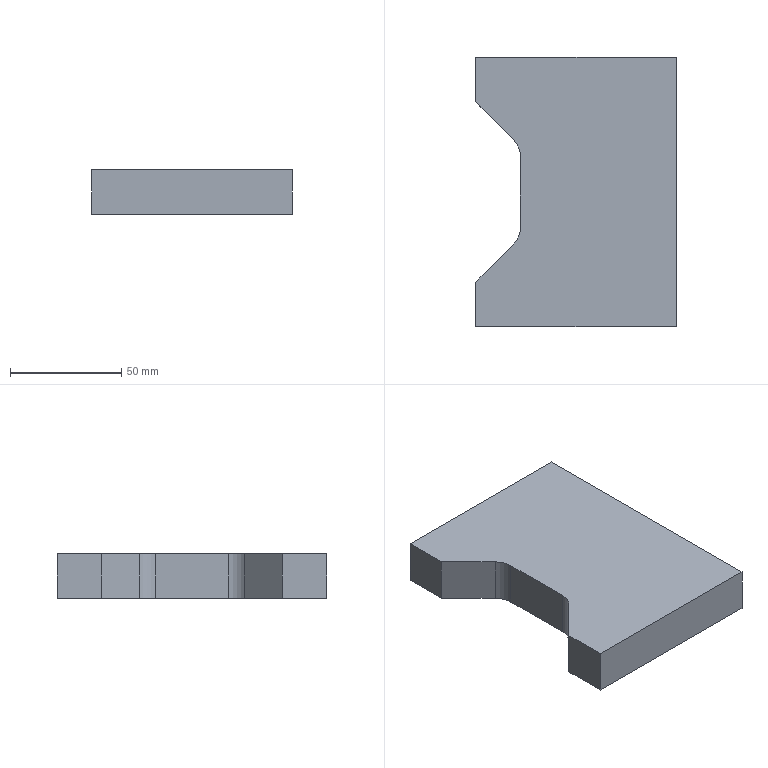Part | SolidWorks | features Extrusion 1 | 1 solid | 12 faces | box 90 x 121 x 20 mm | volume 193486 mm3 | plane 10 | cylinder 2 | commonest cylinder face diameters 20 x2
STEP:
#1=CARTESIAN_POINT('',(0.,0.,0.));
#2=VERTEX_POINT('',#1);
#3=CARTESIAN_POINT('',(0.,-20.,0.));
#4=VERTEX_POINT('',#3);
#5=CARTESIAN_POINT('',(0.,-20.,0.));
#6=DIRECTION('',(0.,-1.,0.));
#7=VECTOR('',#6,1000.);
#8=LINE('',#5,#7);
#9=EDGE_CURVE('',#2,#4,#8,.T.);
#10=ORIENTED_EDGE('',*,*,#9,.T.);
#11=CARTESIAN_POINT('',(0.,-20.,20.));
#12=VERTEX_POINT('',#11);
#13=CARTESIAN_POINT('',(0.,-20.,20.));
#14=DIRECTION('',(0.,0.,-1.));
#15=VECTOR('',#14,1000.);
#16=LINE('',#13,#15);
#17=EDGE_CURVE('',#12,#4,#16,.T.);
#18=ORIENTED_EDGE('',*,*,#17,.F.);
#19=CARTESIAN_POINT('',(0.,0.,20.));
#20=VERTEX_POINT('',#19);
#21=CARTESIAN_POINT('',(0.,-20.,20.));
#22=DIRECTION('',(0.,-1.,0.));
#23=VECTOR('',#22,1000.);
#24=LINE('',#21,#23);
#25=EDGE_CURVE('',#20,#12,#24,.T.);
#26=ORIENTED_EDGE('',*,*,#25,.F.);
#27=CARTESIAN_POINT('',(0.,0.,20.));
#28=DIRECTION('',(0.,0.,-1.));
#29=VECTOR('',#28,1000.);
#30=LINE('',#27,#29);
#31=EDGE_CURVE('',#20,#2,#30,.T.);
#32=ORIENTED_EDGE('',*,*,#31,.T.);
#33=EDGE_LOOP('',(#10,#18,#26,#32));
#34=FACE_OUTER_BOUND('',#33,.T.);
#35=CARTESIAN_POINT('',(0.,-20.,20.));
#36=DIRECTION('',(1.,0.,0.));
#37=DIRECTION('',(0.,0.,-1.));
#38=AXIS2_PLACEMENT_3D('',#35,#36,#37);
#39=PLANE('',#38);
#40=ADVANCED_FACE('',(#34),#39,.F.);
#41=CARTESIAN_POINT('',(17.071,-37.071,0.));
#42=VERTEX_POINT('',#41);
#43=CARTESIAN_POINT('',(17.071,-37.071,0.));
#44=DIRECTION('',(0.7071,-0.7071,0.));
#45=VECTOR('',#44,1000.);
#46=LINE('',#43,#45);
#47=EDGE_CURVE('',#4,#42,#46,.T.);
#48=ORIENTED_EDGE('',*,*,#47,.T.);
#49=CARTESIAN_POINT('',(17.071,-37.071,20.));
#50=VERTEX_POINT('',#49);
#51=CARTESIAN_POINT('',(17.071,-37.071,20.));
#52=DIRECTION('',(0.,0.,-1.));
#53=VECTOR('',#52,1000.);
#54=LINE('',#51,#53);
#55=EDGE_CURVE('',#50,#42,#54,.T.);
#56=ORIENTED_EDGE('',*,*,#55,.F.);
#57=CARTESIAN_POINT('',(17.071,-37.071,20.));
#58=DIRECTION('',(0.7071,-0.7071,0.));
#59=VECTOR('',#58,1000.);
#60=LINE('',#57,#59);
#61=EDGE_CURVE('',#12,#50,#60,.T.);
#62=ORIENTED_EDGE('',*,*,#61,.F.);
#63=ORIENTED_EDGE('',*,*,#17,.T.);
#64=EDGE_LOOP('',(#48,#56,#62,#63));
#65=FACE_OUTER_BOUND('',#64,.T.);
#66=CARTESIAN_POINT('',(17.071,-37.071,20.));
#67=DIRECTION('',(0.7071,0.7071,0.));
#68=DIRECTION('',(-0.7071,0.7071,0.));
#69=AXIS2_PLACEMENT_3D('',#66,#67,#68);
#70=PLANE('',#69);
#71=ADVANCED_FACE('',(#65),#70,.F.);
#72=CARTESIAN_POINT('',(20.,-44.142,0.));
#73=VERTEX_POINT('',#72);
#74=CARTESIAN_POINT('',(10.,-44.142,0.));
#75=DIRECTION('',(0.,0.,-1.));
#76=DIRECTION('',(1.,0.,0.));
#77=AXIS2_PLACEMENT_3D('',#74,#75,#76);
#78=CIRCLE('',#77,10.);
#79=EDGE_CURVE('',#42,#73,#78,.T.);
#80=ORIENTED_EDGE('',*,*,#79,.T.);
#81=CARTESIAN_POINT('',(20.,-44.142,20.));
#82=VERTEX_POINT('',#81);
#83=CARTESIAN_POINT('',(20.,-44.142,20.));
#84=DIRECTION('',(0.,0.,-1.));
#85=VECTOR('',#84,1000.);
#86=LINE('',#83,#85);
#87=EDGE_CURVE('',#82,#73,#86,.T.);
#88=ORIENTED_EDGE('',*,*,#87,.F.);
#89=CARTESIAN_POINT('',(10.,-44.142,20.));
#90=DIRECTION('',(0.,0.,-1.));
#91=DIRECTION('',(1.,0.,0.));
#92=AXIS2_PLACEMENT_3D('',#89,#90,#91);
#93=CIRCLE('',#92,10.);
#94=EDGE_CURVE('',#50,#82,#93,.T.);
#95=ORIENTED_EDGE('',*,*,#94,.F.);
#96=ORIENTED_EDGE('',*,*,#55,.T.);
#97=EDGE_LOOP('',(#80,#88,#95,#96));
#98=FACE_OUTER_BOUND('',#97,.T.);
#99=CARTESIAN_POINT('',(10.,-44.142,20.));
#100=DIRECTION('',(0.,0.,-1.));
#101=DIRECTION('',(-1.,0.,0.));
#102=AXIS2_PLACEMENT_3D('',#99,#100,#101);
#103=CYLINDRICAL_SURFACE('',#102,10.);
#104=ADVANCED_FACE('',(#98),#103,.F.);
#105=CARTESIAN_POINT('',(20.,-76.858,0.));
#106=VERTEX_POINT('',#105);
#107=CARTESIAN_POINT('',(20.,-76.858,0.));
#108=DIRECTION('',(0.,-1.,0.));
#109=VECTOR('',#108,1000.);
#110=LINE('',#107,#109);
#111=EDGE_CURVE('',#73,#106,#110,.T.);
#112=ORIENTED_EDGE('',*,*,#111,.T.);
#113=CARTESIAN_POINT('',(20.,-76.858,20.));
#114=VERTEX_POINT('',#113);
#115=CARTESIAN_POINT('',(20.,-76.858,20.));
#116=DIRECTION('',(0.,0.,-1.));
#117=VECTOR('',#116,1000.);
#118=LINE('',#115,#117);
#119=EDGE_CURVE('',#114,#106,#118,.T.);
#120=ORIENTED_EDGE('',*,*,#119,.F.);
#121=CARTESIAN_POINT('',(20.,-76.858,20.));
#122=DIRECTION('',(0.,-1.,0.));
#123=VECTOR('',#122,1000.);
#124=LINE('',#121,#123);
#125=EDGE_CURVE('',#82,#114,#124,.T.);
#126=ORIENTED_EDGE('',*,*,#125,.F.);
#127=ORIENTED_EDGE('',*,*,#87,.T.);
#128=EDGE_LOOP('',(#112,#120,#126,#127));
#129=FACE_OUTER_BOUND('',#128,.T.);
#130=CARTESIAN_POINT('',(20.,-76.858,20.));
#131=DIRECTION('',(1.,0.,0.));
#132=DIRECTION('',(0.,1.,0.));
#133=AXIS2_PLACEMENT_3D('',#130,#131,#132);
#134=PLANE('',#133);
#135=ADVANCED_FACE('',(#129),#134,.F.);
#136=CARTESIAN_POINT('',(17.071,-83.929,0.));
#137=VERTEX_POINT('',#136);
#138=CARTESIAN_POINT('',(10.,-76.858,0.));
#139=DIRECTION('',(0.,0.,-1.));
#140=DIRECTION('',(1.,0.,0.));
#141=AXIS2_PLACEMENT_3D('',#138,#139,#140);
#142=CIRCLE('',#141,10.);
#143=EDGE_CURVE('',#106,#137,#142,.T.);
#144=ORIENTED_EDGE('',*,*,#143,.T.);
#145=CARTESIAN_POINT('',(17.071,-83.929,20.));
#146=VERTEX_POINT('',#145);
#147=CARTESIAN_POINT('',(17.071,-83.929,20.));
#148=DIRECTION('',(0.,0.,-1.));
#149=VECTOR('',#148,1000.);
#150=LINE('',#147,#149);
#151=EDGE_CURVE('',#146,#137,#150,.T.);
#152=ORIENTED_EDGE('',*,*,#151,.F.);
#153=CARTESIAN_POINT('',(10.,-76.858,20.));
#154=DIRECTION('',(0.,0.,-1.));
#155=DIRECTION('',(1.,0.,0.));
#156=AXIS2_PLACEMENT_3D('',#153,#154,#155);
#157=CIRCLE('',#156,10.);
#158=EDGE_CURVE('',#114,#146,#157,.T.);
#159=ORIENTED_EDGE('',*,*,#158,.F.);
#160=ORIENTED_EDGE('',*,*,#119,.T.);
#161=EDGE_LOOP('',(#144,#152,#159,#160));
#162=FACE_OUTER_BOUND('',#161,.T.);
#163=CARTESIAN_POINT('',(10.,-76.858,20.));
#164=DIRECTION('',(0.,0.,-1.));
#165=DIRECTION('',(-1.,0.,0.));
#166=AXIS2_PLACEMENT_3D('',#163,#164,#165);
#167=CYLINDRICAL_SURFACE('',#166,10.);
#168=ADVANCED_FACE('',(#162),#167,.F.);
#169=CARTESIAN_POINT('',(0.,-101.,0.));
#170=VERTEX_POINT('',#169);
#171=CARTESIAN_POINT('',(0.,-101.,0.));
#172=DIRECTION('',(-0.7071,-0.7071,0.));
#173=VECTOR('',#172,1000.);
#174=LINE('',#171,#173);
#175=EDGE_CURVE('',#137,#170,#174,.T.);
#176=ORIENTED_EDGE('',*,*,#175,.T.);
#177=CARTESIAN_POINT('',(0.,-101.,20.));
#178=VERTEX_POINT('',#177);
#179=CARTESIAN_POINT('',(0.,-101.,20.));
#180=DIRECTION('',(0.,0.,-1.));
#181=VECTOR('',#180,1000.);
#182=LINE('',#179,#181);
#183=EDGE_CURVE('',#178,#170,#182,.T.);
#184=ORIENTED_EDGE('',*,*,#183,.F.);
#185=CARTESIAN_POINT('',(0.,-101.,20.));
#186=DIRECTION('',(-0.7071,-0.7071,0.));
#187=VECTOR('',#186,1000.);
#188=LINE('',#185,#187);
#189=EDGE_CURVE('',#146,#178,#188,.T.);
#190=ORIENTED_EDGE('',*,*,#189,.F.);
#191=ORIENTED_EDGE('',*,*,#151,.T.);
#192=EDGE_LOOP('',(#176,#184,#190,#191));
#193=FACE_OUTER_BOUND('',#192,.T.);
#194=CARTESIAN_POINT('',(0.,-101.,20.));
#195=DIRECTION('',(0.7071,-0.7071,0.));
#196=DIRECTION('',(0.7071,0.7071,0.));
#197=AXIS2_PLACEMENT_3D('',#194,#195,#196);
#198=PLANE('',#197);
#199=ADVANCED_FACE('',(#193),#198,.F.);
#200=CARTESIAN_POINT('',(0.,-121.,0.));
#201=VERTEX_POINT('',#200);
#202=CARTESIAN_POINT('',(0.,-121.,0.));
#203=DIRECTION('',(0.,-1.,0.));
#204=VECTOR('',#203,1000.);
#205=LINE('',#202,#204);
#206=EDGE_CURVE('',#170,#201,#205,.T.);
#207=ORIENTED_EDGE('',*,*,#206,.T.);
#208=CARTESIAN_POINT('',(0.,-121.,20.));
#209=VERTEX_POINT('',#208);
#210=CARTESIAN_POINT('',(0.,-121.,20.));
#211=DIRECTION('',(0.,0.,-1.));
#212=VECTOR('',#211,1000.);
#213=LINE('',#210,#212);
#214=EDGE_CURVE('',#209,#201,#213,.T.);
#215=ORIENTED_EDGE('',*,*,#214,.F.);
#216=CARTESIAN_POINT('',(0.,-121.,20.));
#217=DIRECTION('',(0.,-1.,0.));
#218=VECTOR('',#217,1000.);
#219=LINE('',#216,#218);
#220=EDGE_CURVE('',#178,#209,#219,.T.);
#221=ORIENTED_EDGE('',*,*,#220,.F.);
#222=ORIENTED_EDGE('',*,*,#183,.T.);
#223=EDGE_LOOP('',(#207,#215,#221,#222));
#224=FACE_OUTER_BOUND('',#223,.T.);
#225=CARTESIAN_POINT('',(0.,-121.,20.));
#226=DIRECTION('',(1.,0.,0.));
#227=DIRECTION('',(0.,1.,0.));
#228=AXIS2_PLACEMENT_3D('',#225,#226,#227);
#229=PLANE('',#228);
#230=ADVANCED_FACE('',(#224),#229,.F.);
#231=CARTESIAN_POINT('',(90.,-121.,0.));
#232=VERTEX_POINT('',#231);
#233=CARTESIAN_POINT('',(90.,-121.,0.));
#234=DIRECTION('',(1.,0.,0.));
#235=VECTOR('',#234,1000.);
#236=LINE('',#233,#235);
#237=EDGE_CURVE('',#201,#232,#236,.T.);
#238=ORIENTED_EDGE('',*,*,#237,.T.);
#239=CARTESIAN_POINT('',(90.,-121.,20.));
#240=VERTEX_POINT('',#239);
#241=CARTESIAN_POINT('',(90.,-121.,20.));
#242=DIRECTION('',(0.,0.,-1.));
#243=VECTOR('',#242,1000.);
#244=LINE('',#241,#243);
#245=EDGE_CURVE('',#240,#232,#244,.T.);
#246=ORIENTED_EDGE('',*,*,#245,.F.);
#247=CARTESIAN_POINT('',(90.,-121.,20.));
#248=DIRECTION('',(1.,0.,0.));
#249=VECTOR('',#248,1000.);
#250=LINE('',#247,#249);
#251=EDGE_CURVE('',#209,#240,#250,.T.);
#252=ORIENTED_EDGE('',*,*,#251,.F.);
#253=ORIENTED_EDGE('',*,*,#214,.T.);
#254=EDGE_LOOP('',(#238,#246,#252,#253));
#255=FACE_OUTER_BOUND('',#254,.T.);
#256=CARTESIAN_POINT('',(90.,-121.,20.));
#257=DIRECTION('',(0.,1.,0.));
#258=DIRECTION('',(-1.,0.,0.));
#259=AXIS2_PLACEMENT_3D('',#256,#257,#258);
#260=PLANE('',#259);
#261=ADVANCED_FACE('',(#255),#260,.F.);
#262=CARTESIAN_POINT('',(90.,0.,0.));
#263=VERTEX_POINT('',#262);
#264=CARTESIAN_POINT('',(90.,0.,0.));
#265=DIRECTION('',(0.,1.,0.));
#266=VECTOR('',#265,1000.);
#267=LINE('',#264,#266);
#268=EDGE_CURVE('',#232,#263,#267,.T.);
#269=ORIENTED_EDGE('',*,*,#268,.T.);
#270=CARTESIAN_POINT('',(90.,0.,20.));
#271=VERTEX_POINT('',#270);
#272=CARTESIAN_POINT('',(90.,0.,20.));
#273=DIRECTION('',(0.,0.,-1.));
#274=VECTOR('',#273,1000.);
#275=LINE('',#272,#274);
#276=EDGE_CURVE('',#271,#263,#275,.T.);
#277=ORIENTED_EDGE('',*,*,#276,.F.);
#278=CARTESIAN_POINT('',(90.,0.,20.));
#279=DIRECTION('',(0.,1.,0.));
#280=VECTOR('',#279,1000.);
#281=LINE('',#278,#280);
#282=EDGE_CURVE('',#240,#271,#281,.T.);
#283=ORIENTED_EDGE('',*,*,#282,.F.);
#284=ORIENTED_EDGE('',*,*,#245,.T.);
#285=EDGE_LOOP('',(#269,#277,#283,#284));
#286=FACE_OUTER_BOUND('',#285,.T.);
#287=CARTESIAN_POINT('',(90.,0.,20.));
#288=DIRECTION('',(-1.,0.,0.));
#289=DIRECTION('',(0.,-1.,0.));
#290=AXIS2_PLACEMENT_3D('',#287,#288,#289);
#291=PLANE('',#290);
#292=ADVANCED_FACE('',(#286),#291,.F.);
#293=CARTESIAN_POINT('',(0.,0.,0.));
#294=DIRECTION('',(-1.,0.,0.));
#295=VECTOR('',#294,1000.);
#296=LINE('',#293,#295);
#297=EDGE_CURVE('',#263,#2,#296,.T.);
#298=ORIENTED_EDGE('',*,*,#297,.T.);
#299=ORIENTED_EDGE('',*,*,#31,.F.);
#300=CARTESIAN_POINT('',(0.,0.,20.));
#301=DIRECTION('',(-1.,0.,0.));
#302=VECTOR('',#301,1000.);
#303=LINE('',#300,#302);
#304=EDGE_CURVE('',#271,#20,#303,.T.);
#305=ORIENTED_EDGE('',*,*,#304,.F.);
#306=ORIENTED_EDGE('',*,*,#276,.T.);
#307=EDGE_LOOP('',(#298,#299,#305,#306));
#308=FACE_OUTER_BOUND('',#307,.T.);
#309=CARTESIAN_POINT('',(0.,0.,20.));
#310=DIRECTION('',(0.,-1.,0.));
#311=DIRECTION('',(0.,0.,-1.));
#312=AXIS2_PLACEMENT_3D('',#309,#310,#311);
#313=PLANE('',#312);
#314=ADVANCED_FACE('',(#308),#313,.F.);
#315=ORIENTED_EDGE('',*,*,#25,.T.);
#316=ORIENTED_EDGE('',*,*,#61,.T.);
#317=ORIENTED_EDGE('',*,*,#94,.T.);
#318=ORIENTED_EDGE('',*,*,#125,.T.);
#319=ORIENTED_EDGE('',*,*,#158,.T.);
#320=ORIENTED_EDGE('',*,*,#189,.T.);
#321=ORIENTED_EDGE('',*,*,#220,.T.);
#322=ORIENTED_EDGE('',*,*,#251,.T.);
#323=ORIENTED_EDGE('',*,*,#282,.T.);
#324=ORIENTED_EDGE('',*,*,#304,.T.);
#325=EDGE_LOOP('',(#315,#316,#317,#318,#319,#320,#321,#322,#323,#324));
#326=FACE_OUTER_BOUND('',#325,.T.);
#327=CARTESIAN_POINT('',(10.,-76.858,20.));
#328=DIRECTION('',(0.,0.,1.));
#329=DIRECTION('',(1.,0.,0.));
#330=AXIS2_PLACEMENT_3D('',#327,#328,#329);
#331=PLANE('',#330);
#332=ADVANCED_FACE('',(#326),#331,.T.);
#333=ORIENTED_EDGE('',*,*,#9,.F.);
#334=ORIENTED_EDGE('',*,*,#297,.F.);
#335=ORIENTED_EDGE('',*,*,#268,.F.);
#336=ORIENTED_EDGE('',*,*,#237,.F.);
#337=ORIENTED_EDGE('',*,*,#206,.F.);
#338=ORIENTED_EDGE('',*,*,#175,.F.);
#339=ORIENTED_EDGE('',*,*,#143,.F.);
#340=ORIENTED_EDGE('',*,*,#111,.F.);
#341=ORIENTED_EDGE('',*,*,#79,.F.);
#342=ORIENTED_EDGE('',*,*,#47,.F.);
#343=EDGE_LOOP('',(#333,#334,#335,#336,#337,#338,#339,#340,#341,#342));
#344=FACE_OUTER_BOUND('',#343,.T.);
#345=CARTESIAN_POINT('',(10.,-76.858,0.));
#346=DIRECTION('',(0.,0.,1.));
#347=DIRECTION('',(1.,0.,0.));
#348=AXIS2_PLACEMENT_3D('',#345,#346,#347);
#349=PLANE('',#348);
#350=ADVANCED_FACE('',(#344),#349,.F.);
#351=CLOSED_SHELL('',(#40,#71,#104,#135,#168,#199,#230,#261,#292,#314,#332,#350));
#352=MANIFOLD_SOLID_BREP('',#351);
#353=CARTESIAN_POINT('',(0.,0.,0.));
#354=DIRECTION('',(0.,0.,1.));
#355=DIRECTION('',(1.,0.,0.));
#356=AXIS2_PLACEMENT_3D('',#353,#354,#355);
#357=(LENGTH_UNIT()NAMED_UNIT(*)SI_UNIT(.MILLI.,.METRE.));
#358=UNCERTAINTY_MEASURE_WITH_UNIT(LENGTH_MEASURE(0.00001),#357,'','');
#359=(NAMED_UNIT(*)PLANE_ANGLE_UNIT()SI_UNIT($,.RADIAN.));
#360=(NAMED_UNIT(*)SI_UNIT($,.STERADIAN.)SOLID_ANGLE_UNIT());
#361=(GEOMETRIC_REPRESENTATION_CONTEXT(3)GLOBAL_UNCERTAINTY_ASSIGNED_CONTEXT((#358))GLOBAL_UNIT_ASSIGNED_CONTEXT((#357,#359,#360))REPRESENTATION_CONTEXT('',''));
#362=ADVANCED_BREP_SHAPE_REPRESENTATION('',(#352,#356),#361);